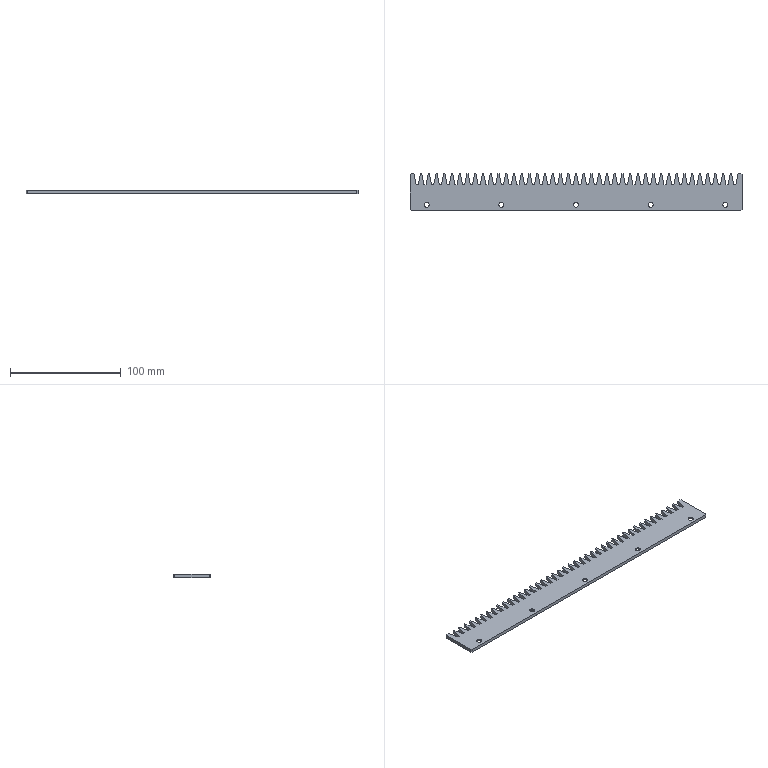Part | SolidWorks | features Chamfer 1, Extrusion 1, HoleWzd 1, ICE 1 | 1 solid | 198 faces | box 300 x 33 x 3 mm | volume 24182 mm3 | plane 178 | cone 10 | cylinder 10 | commonest cylinder face diameters 4.5 x10